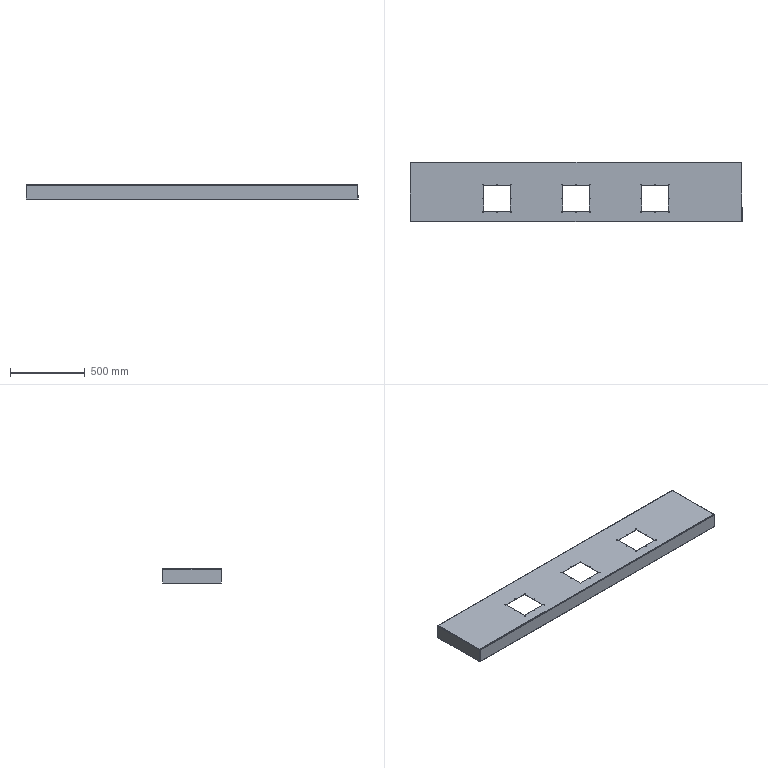Part | SolidWorks | features EdgeFlange 2, FlatPattern 1, SMBaseFlange 1, SheetMetal 1 | 1 solid | 142 faces | box 2224 x 400.113 x 100 mm | volume 2783489 mm3 | cylinder 76 | plane 50 | spline 16 | commonest cylinder face diameters 5.4 x48 4 x16 1.473 x4 5.473 x4 8 x4